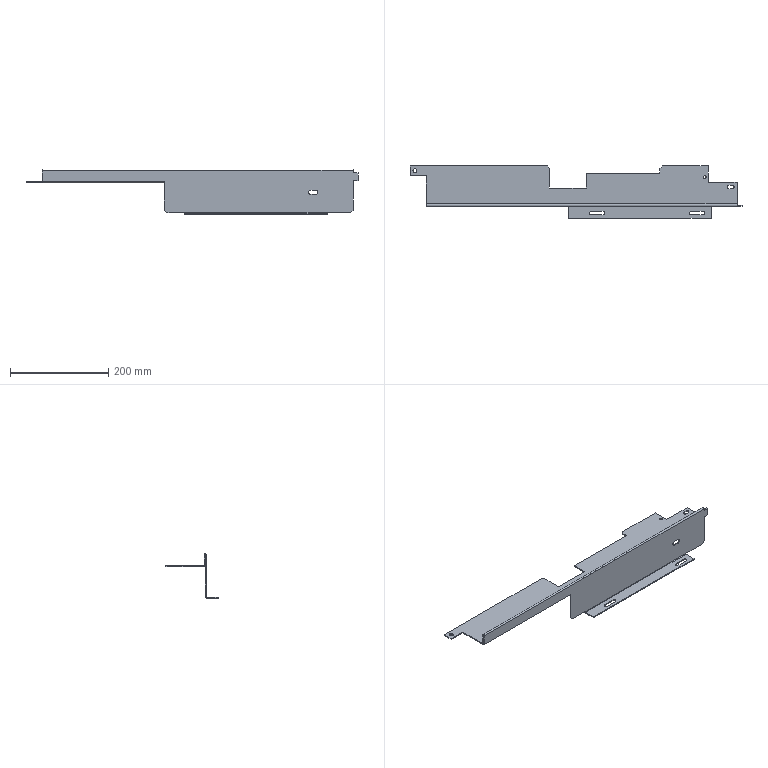Part | STEP file | 1 solid | 69 faces | box 676 x 106.1 x 90 mm | volume 208424 mm3 | plane 48 | cylinder 21 | commonest cylinder face diameters 7 x9 6 x4 2 x2 8 x2 9 x2 0.1 x1